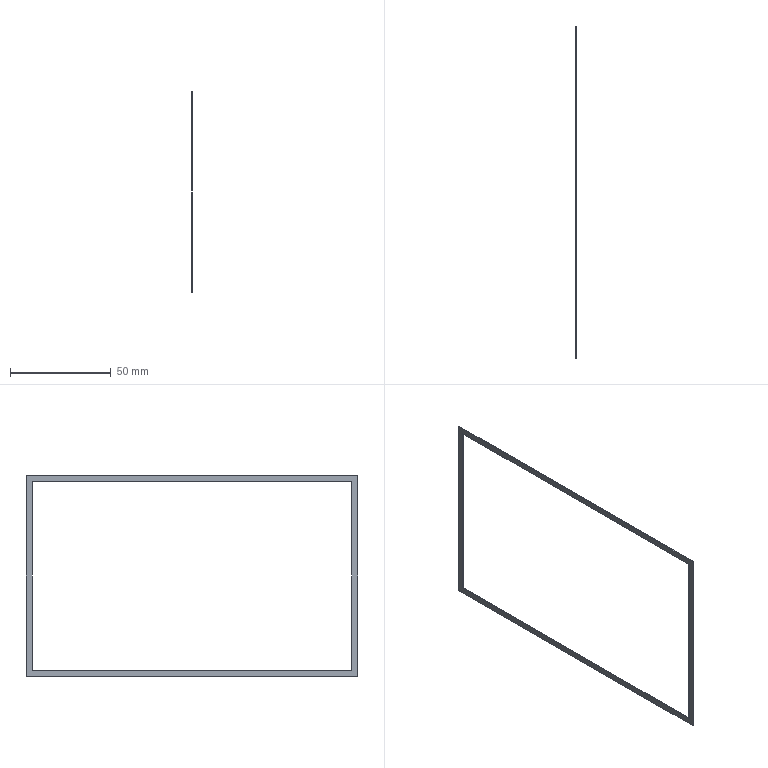Part | STEP file | 1 solid | 10 faces | box 0.3 x 164.6 x 99.7 mm | volume 464.94 mm3 | plane 10
STEP:
#1=CARTESIAN_POINT('',(0.,0.,0.));
#2=DIRECTION('',(0.,0.,1.));
#3=DIRECTION('',(1.,0.,0.));
#4=AXIS2_PLACEMENT_3D('',#1,#2,#3);
#5=CARTESIAN_POINT('',(769.075,4084.39,1378.984));
#6=VERTEX_POINT('',#5);
#7=CARTESIAN_POINT('',(769.075,4084.39,1285.284));
#8=VERTEX_POINT('',#7);
#9=CARTESIAN_POINT('',(769.075,4084.39,1378.984));
#10=DIRECTION('',(0.,0.,-1.));
#11=VECTOR('',#10,1.);
#12=LINE('',#9,#11);
#13=CARTESIAN_POINT('',(769.375,4084.39,1285.284));
#14=DIRECTION('',(0.,-1.,0.));
#15=DIRECTION('',(0.,0.,-1.));
#16=AXIS2_PLACEMENT_3D('',#13,#14,#15);
#17=PLANE('',#16);
#18=CARTESIAN_POINT('',(-93.7,-0.3));
#19=DIRECTION('',(1.,0.));
#20=VECTOR('',#19,1.);
#21=LINE('',#18,#20);
#22=(GEOMETRIC_REPRESENTATION_CONTEXT(2)PARAMETRIC_REPRESENTATION_CONTEXT()REPRESENTATION_CONTEXT('',''));
#23=DEFINITIONAL_REPRESENTATION('',(#21),#22);
#24=PCURVE('',#17,#23);
#25=CARTESIAN_POINT('',(769.075,0.,0.));
#26=DIRECTION('',(1.,0.,0.));
#27=DIRECTION('',(0.,0.,-1.));
#28=AXIS2_PLACEMENT_3D('',#25,#26,#27);
#29=PLANE('',#28);
#30=CARTESIAN_POINT('',(-1378.984,4084.39));
#31=DIRECTION('',(1.,0.));
#32=VECTOR('',#31,1.);
#33=LINE('',#30,#32);
#34=(GEOMETRIC_REPRESENTATION_CONTEXT(2)PARAMETRIC_REPRESENTATION_CONTEXT()REPRESENTATION_CONTEXT('',''));
#35=DEFINITIONAL_REPRESENTATION('',(#33),#34);
#36=PCURVE('',#29,#35);
#37=SURFACE_CURVE('',#12,(#24,#36),.PCURVE_S1.);
#38=EDGE_CURVE('',#6,#8,#37,.T.);
#39=ORIENTED_EDGE('',*,*,#38,.T.);
#40=CARTESIAN_POINT('',(769.375,4084.39,1285.284));
#41=VERTEX_POINT('',#40);
#42=CARTESIAN_POINT('',(769.075,4084.39,1285.284));
#43=DIRECTION('',(1.,0.,0.));
#44=VECTOR('',#43,1.);
#45=LINE('',#42,#44);
#46=CARTESIAN_POINT('',(0.,-0.3));
#47=DIRECTION('',(0.,1.));
#48=VECTOR('',#47,1.);
#49=LINE('',#46,#48);
#50=(GEOMETRIC_REPRESENTATION_CONTEXT(2)PARAMETRIC_REPRESENTATION_CONTEXT()REPRESENTATION_CONTEXT('',''));
#51=DEFINITIONAL_REPRESENTATION('',(#49),#50);
#52=PCURVE('',#17,#51);
#53=CARTESIAN_POINT('',(769.375,4242.99,1285.284));
#54=DIRECTION('',(0.,0.,-1.));
#55=DIRECTION('',(-1.,0.,0.));
#56=AXIS2_PLACEMENT_3D('',#53,#54,#55);
#57=PLANE('',#56);
#58=CARTESIAN_POINT('',(0.3,-158.6));
#59=DIRECTION('',(-1.,0.));
#60=VECTOR('',#59,1.);
#61=LINE('',#58,#60);
#62=(GEOMETRIC_REPRESENTATION_CONTEXT(2)PARAMETRIC_REPRESENTATION_CONTEXT()REPRESENTATION_CONTEXT('',''));
#63=DEFINITIONAL_REPRESENTATION('',(#61),#62);
#64=PCURVE('',#57,#63);
#65=SURFACE_CURVE('',#45,(#52,#64),.PCURVE_S1.);
#66=EDGE_CURVE('',#8,#41,#65,.T.);
#67=ORIENTED_EDGE('',*,*,#66,.T.);
#68=CARTESIAN_POINT('',(769.375,4084.39,1378.984));
#69=VERTEX_POINT('',#68);
#70=CARTESIAN_POINT('',(769.375,4084.39,1378.984));
#71=DIRECTION('',(0.,0.,-1.));
#72=VECTOR('',#71,1.);
#73=LINE('',#70,#72);
#74=CARTESIAN_POINT('',(-93.7,0.));
#75=DIRECTION('',(1.,0.));
#76=VECTOR('',#75,1.);
#77=LINE('',#74,#76);
#78=(GEOMETRIC_REPRESENTATION_CONTEXT(2)PARAMETRIC_REPRESENTATION_CONTEXT()REPRESENTATION_CONTEXT('',''));
#79=DEFINITIONAL_REPRESENTATION('',(#77),#78);
#80=PCURVE('',#17,#79);
#81=CARTESIAN_POINT('',(769.375,0.,0.));
#82=DIRECTION('',(1.,0.,0.));
#83=DIRECTION('',(0.,0.,-1.));
#84=AXIS2_PLACEMENT_3D('',#81,#82,#83);
#85=PLANE('',#84);
#86=CARTESIAN_POINT('',(-1378.984,4084.39));
#87=DIRECTION('',(1.,0.));
#88=VECTOR('',#87,1.);
#89=LINE('',#86,#88);
#90=(GEOMETRIC_REPRESENTATION_CONTEXT(2)PARAMETRIC_REPRESENTATION_CONTEXT()REPRESENTATION_CONTEXT('',''));
#91=DEFINITIONAL_REPRESENTATION('',(#89),#90);
#92=PCURVE('',#85,#91);
#93=SURFACE_CURVE('',#73,(#80,#92),.PCURVE_S1.);
#94=EDGE_CURVE('',#69,#41,#93,.T.);
#95=ORIENTED_EDGE('',*,*,#94,.F.);
#96=CARTESIAN_POINT('',(769.075,4084.39,1378.984));
#97=DIRECTION('',(1.,0.,0.));
#98=VECTOR('',#97,1.);
#99=LINE('',#96,#98);
#100=CARTESIAN_POINT('',(-93.7,-0.3));
#101=DIRECTION('',(0.,1.));
#102=VECTOR('',#101,1.);
#103=LINE('',#100,#102);
#104=(GEOMETRIC_REPRESENTATION_CONTEXT(2)PARAMETRIC_REPRESENTATION_CONTEXT()REPRESENTATION_CONTEXT('',''));
#105=DEFINITIONAL_REPRESENTATION('',(#103),#104);
#106=PCURVE('',#17,#105);
#107=CARTESIAN_POINT('',(769.375,4084.39,1378.984));
#108=DIRECTION('',(0.,0.,1.));
#109=DIRECTION('',(1.,0.,0.));
#110=AXIS2_PLACEMENT_3D('',#107,#108,#109);
#111=PLANE('',#110);
#112=CARTESIAN_POINT('',(-0.3,0.));
#113=DIRECTION('',(1.,0.));
#114=VECTOR('',#113,1.);
#115=LINE('',#112,#114);
#116=(GEOMETRIC_REPRESENTATION_CONTEXT(2)PARAMETRIC_REPRESENTATION_CONTEXT()REPRESENTATION_CONTEXT('',''));
#117=DEFINITIONAL_REPRESENTATION('',(#115),#116);
#118=PCURVE('',#111,#117);
#119=SURFACE_CURVE('',#99,(#106,#118),.PCURVE_S1.);
#120=EDGE_CURVE('',#6,#69,#119,.T.);
#121=ORIENTED_EDGE('',*,*,#120,.F.);
#122=EDGE_LOOP('',(#39,#67,#95,#121));
#123=FACE_BOUND('',#122,.F.);
#124=ADVANCED_FACE('',(#123),#17,.F.);
#125=CARTESIAN_POINT('',(769.075,4081.39,1282.284));
#126=VERTEX_POINT('',#125);
#127=CARTESIAN_POINT('',(769.075,4081.39,1381.984));
#128=VERTEX_POINT('',#127);
#129=CARTESIAN_POINT('',(769.075,4081.39,1282.284));
#130=DIRECTION('',(0.,0.,1.));
#131=VECTOR('',#130,1.);
#132=LINE('',#129,#131);
#133=CARTESIAN_POINT('',(-1282.284,4081.39));
#134=DIRECTION('',(-1.,0.));
#135=VECTOR('',#134,1.);
#136=LINE('',#133,#135);
#137=(GEOMETRIC_REPRESENTATION_CONTEXT(2)PARAMETRIC_REPRESENTATION_CONTEXT()REPRESENTATION_CONTEXT('',''));
#138=DEFINITIONAL_REPRESENTATION('',(#136),#137);
#139=PCURVE('',#29,#138);
#140=CARTESIAN_POINT('',(769.375,4081.39,1381.984));
#141=DIRECTION('',(0.,1.,0.));
#142=DIRECTION('',(0.,0.,1.));
#143=AXIS2_PLACEMENT_3D('',#140,#141,#142);
#144=PLANE('',#143);
#145=CARTESIAN_POINT('',(-99.7,-0.3));
#146=DIRECTION('',(1.,0.));
#147=VECTOR('',#146,1.);
#148=LINE('',#145,#147);
#149=(GEOMETRIC_REPRESENTATION_CONTEXT(2)PARAMETRIC_REPRESENTATION_CONTEXT()REPRESENTATION_CONTEXT('',''));
#150=DEFINITIONAL_REPRESENTATION('',(#148),#149);
#151=PCURVE('',#144,#150);
#152=SURFACE_CURVE('',#132,(#139,#151),.PCURVE_S1.);
#153=EDGE_CURVE('',#126,#128,#152,.T.);
#154=ORIENTED_EDGE('',*,*,#153,.F.);
#155=CARTESIAN_POINT('',(769.075,4245.99,1282.284));
#156=VERTEX_POINT('',#155);
#157=CARTESIAN_POINT('',(769.075,4245.99,1282.284));
#158=DIRECTION('',(0.,-1.,0.));
#159=VECTOR('',#158,1.);
#160=LINE('',#157,#159);
#161=CARTESIAN_POINT('',(-1282.284,4245.99));
#162=DIRECTION('',(0.,-1.));
#163=VECTOR('',#162,1.);
#164=LINE('',#161,#163);
#165=(GEOMETRIC_REPRESENTATION_CONTEXT(2)PARAMETRIC_REPRESENTATION_CONTEXT()REPRESENTATION_CONTEXT('',''));
#166=DEFINITIONAL_REPRESENTATION('',(#164),#165);
#167=PCURVE('',#29,#166);
#168=CARTESIAN_POINT('',(769.375,4081.39,1282.284));
#169=DIRECTION('',(0.,0.,1.));
#170=DIRECTION('',(1.,0.,0.));
#171=AXIS2_PLACEMENT_3D('',#168,#169,#170);
#172=PLANE('',#171);
#173=CARTESIAN_POINT('',(-0.3,164.6));
#174=DIRECTION('',(0.,-1.));
#175=VECTOR('',#174,1.);
#176=LINE('',#173,#175);
#177=(GEOMETRIC_REPRESENTATION_CONTEXT(2)PARAMETRIC_REPRESENTATION_CONTEXT()REPRESENTATION_CONTEXT('',''));
#178=DEFINITIONAL_REPRESENTATION('',(#176),#177);
#179=PCURVE('',#172,#178);
#180=SURFACE_CURVE('',#160,(#167,#179),.PCURVE_S1.);
#181=EDGE_CURVE('',#156,#126,#180,.T.);
#182=ORIENTED_EDGE('',*,*,#181,.F.);
#183=CARTESIAN_POINT('',(769.075,4245.99,1381.984));
#184=VERTEX_POINT('',#183);
#185=CARTESIAN_POINT('',(769.075,4245.99,1381.984));
#186=DIRECTION('',(0.,0.,-1.));
#187=VECTOR('',#186,1.);
#188=LINE('',#185,#187);
#189=CARTESIAN_POINT('',(-1381.984,4245.99));
#190=DIRECTION('',(1.,0.));
#191=VECTOR('',#190,1.);
#192=LINE('',#189,#191);
#193=(GEOMETRIC_REPRESENTATION_CONTEXT(2)PARAMETRIC_REPRESENTATION_CONTEXT()REPRESENTATION_CONTEXT('',''));
#194=DEFINITIONAL_REPRESENTATION('',(#192),#193);
#195=PCURVE('',#29,#194);
#196=CARTESIAN_POINT('',(769.375,4245.99,1282.284));
#197=DIRECTION('',(0.,-1.,0.));
#198=DIRECTION('',(0.,0.,-1.));
#199=AXIS2_PLACEMENT_3D('',#196,#197,#198);
#200=PLANE('',#199);
#201=CARTESIAN_POINT('',(-99.7,-0.3));
#202=DIRECTION('',(1.,0.));
#203=VECTOR('',#202,1.);
#204=LINE('',#201,#203);
#205=(GEOMETRIC_REPRESENTATION_CONTEXT(2)PARAMETRIC_REPRESENTATION_CONTEXT()REPRESENTATION_CONTEXT('',''));
#206=DEFINITIONAL_REPRESENTATION('',(#204),#205);
#207=PCURVE('',#200,#206);
#208=SURFACE_CURVE('',#188,(#195,#207),.PCURVE_S1.);
#209=EDGE_CURVE('',#184,#156,#208,.T.);
#210=ORIENTED_EDGE('',*,*,#209,.F.);
#211=CARTESIAN_POINT('',(769.075,4081.39,1381.984));
#212=DIRECTION('',(0.,1.,0.));
#213=VECTOR('',#212,1.);
#214=LINE('',#211,#213);
#215=CARTESIAN_POINT('',(-1381.984,4081.39));
#216=DIRECTION('',(0.,1.));
#217=VECTOR('',#216,1.);
#218=LINE('',#215,#217);
#219=(GEOMETRIC_REPRESENTATION_CONTEXT(2)PARAMETRIC_REPRESENTATION_CONTEXT()REPRESENTATION_CONTEXT('',''));
#220=DEFINITIONAL_REPRESENTATION('',(#218),#219);
#221=PCURVE('',#29,#220);
#222=CARTESIAN_POINT('',(769.375,4245.99,1381.984));
#223=DIRECTION('',(0.,0.,-1.));
#224=DIRECTION('',(-1.,0.,0.));
#225=AXIS2_PLACEMENT_3D('',#222,#223,#224);
#226=PLANE('',#225);
#227=CARTESIAN_POINT('',(0.3,-164.6));
#228=DIRECTION('',(0.,1.));
#229=VECTOR('',#228,1.);
#230=LINE('',#227,#229);
#231=(GEOMETRIC_REPRESENTATION_CONTEXT(2)PARAMETRIC_REPRESENTATION_CONTEXT()REPRESENTATION_CONTEXT('',''));
#232=DEFINITIONAL_REPRESENTATION('',(#230),#231);
#233=PCURVE('',#226,#232);
#234=SURFACE_CURVE('',#214,(#221,#233),.PCURVE_S1.);
#235=EDGE_CURVE('',#128,#184,#234,.T.);
#236=ORIENTED_EDGE('',*,*,#235,.F.);
#237=EDGE_LOOP('',(#154,#182,#210,#236));
#238=FACE_BOUND('',#237,.F.);
#239=ORIENTED_EDGE('',*,*,#38,.F.);
#240=CARTESIAN_POINT('',(769.075,4242.99,1378.984));
#241=VERTEX_POINT('',#240);
#242=CARTESIAN_POINT('',(769.075,4242.99,1378.984));
#243=DIRECTION('',(0.,-1.,0.));
#244=VECTOR('',#243,1.);
#245=LINE('',#242,#244);
#246=CARTESIAN_POINT('',(-1378.984,4242.99));
#247=DIRECTION('',(0.,-1.));
#248=VECTOR('',#247,1.);
#249=LINE('',#246,#248);
#250=(GEOMETRIC_REPRESENTATION_CONTEXT(2)PARAMETRIC_REPRESENTATION_CONTEXT()REPRESENTATION_CONTEXT('',''));
#251=DEFINITIONAL_REPRESENTATION('',(#249),#250);
#252=PCURVE('',#29,#251);
#253=CARTESIAN_POINT('',(-0.3,158.6));
#254=DIRECTION('',(0.,-1.));
#255=VECTOR('',#254,1.);
#256=LINE('',#253,#255);
#257=(GEOMETRIC_REPRESENTATION_CONTEXT(2)PARAMETRIC_REPRESENTATION_CONTEXT()REPRESENTATION_CONTEXT('',''));
#258=DEFINITIONAL_REPRESENTATION('',(#256),#257);
#259=PCURVE('',#111,#258);
#260=SURFACE_CURVE('',#245,(#252,#259),.PCURVE_S1.);
#261=EDGE_CURVE('',#241,#6,#260,.T.);
#262=ORIENTED_EDGE('',*,*,#261,.F.);
#263=CARTESIAN_POINT('',(769.075,4242.99,1285.284));
#264=VERTEX_POINT('',#263);
#265=CARTESIAN_POINT('',(769.075,4242.99,1285.284));
#266=DIRECTION('',(0.,0.,1.));
#267=VECTOR('',#266,1.);
#268=LINE('',#265,#267);
#269=CARTESIAN_POINT('',(-1285.284,4242.99));
#270=DIRECTION('',(-1.,0.));
#271=VECTOR('',#270,1.);
#272=LINE('',#269,#271);
#273=(GEOMETRIC_REPRESENTATION_CONTEXT(2)PARAMETRIC_REPRESENTATION_CONTEXT()REPRESENTATION_CONTEXT('',''));
#274=DEFINITIONAL_REPRESENTATION('',(#272),#273);
#275=PCURVE('',#29,#274);
#276=CARTESIAN_POINT('',(769.375,4242.99,1378.984));
#277=DIRECTION('',(0.,1.,0.));
#278=DIRECTION('',(0.,0.,1.));
#279=AXIS2_PLACEMENT_3D('',#276,#277,#278);
#280=PLANE('',#279);
#281=CARTESIAN_POINT('',(-93.7,-0.3));
#282=DIRECTION('',(1.,0.));
#283=VECTOR('',#282,1.);
#284=LINE('',#281,#283);
#285=(GEOMETRIC_REPRESENTATION_CONTEXT(2)PARAMETRIC_REPRESENTATION_CONTEXT()REPRESENTATION_CONTEXT('',''));
#286=DEFINITIONAL_REPRESENTATION('',(#284),#285);
#287=PCURVE('',#280,#286);
#288=SURFACE_CURVE('',#268,(#275,#287),.PCURVE_S1.);
#289=EDGE_CURVE('',#264,#241,#288,.T.);
#290=ORIENTED_EDGE('',*,*,#289,.F.);
#291=CARTESIAN_POINT('',(769.075,4084.39,1285.284));
#292=DIRECTION('',(0.,1.,0.));
#293=VECTOR('',#292,1.);
#294=LINE('',#291,#293);
#295=CARTESIAN_POINT('',(-1285.284,4084.39));
#296=DIRECTION('',(0.,1.));
#297=VECTOR('',#296,1.);
#298=LINE('',#295,#297);
#299=(GEOMETRIC_REPRESENTATION_CONTEXT(2)PARAMETRIC_REPRESENTATION_CONTEXT()REPRESENTATION_CONTEXT('',''));
#300=DEFINITIONAL_REPRESENTATION('',(#298),#299);
#301=PCURVE('',#29,#300);
#302=CARTESIAN_POINT('',(0.3,-158.6));
#303=DIRECTION('',(0.,1.));
#304=VECTOR('',#303,1.);
#305=LINE('',#302,#304);
#306=(GEOMETRIC_REPRESENTATION_CONTEXT(2)PARAMETRIC_REPRESENTATION_CONTEXT()REPRESENTATION_CONTEXT('',''));
#307=DEFINITIONAL_REPRESENTATION('',(#305),#306);
#308=PCURVE('',#57,#307);
#309=SURFACE_CURVE('',#294,(#301,#308),.PCURVE_S1.);
#310=EDGE_CURVE('',#8,#264,#309,.T.);
#311=ORIENTED_EDGE('',*,*,#310,.F.);
#312=EDGE_LOOP('',(#239,#262,#290,#311));
#313=FACE_BOUND('',#312,.F.);
#314=ADVANCED_FACE('',(#238,#313),#29,.F.);
#315=ORIENTED_EDGE('',*,*,#153,.T.);
#316=CARTESIAN_POINT('',(769.375,4081.39,1381.984));
#317=VERTEX_POINT('',#316);
#318=CARTESIAN_POINT('',(769.075,4081.39,1381.984));
#319=DIRECTION('',(1.,0.,0.));
#320=VECTOR('',#319,1.);
#321=LINE('',#318,#320);
#322=CARTESIAN_POINT('',(0.,-0.3));
#323=DIRECTION('',(0.,1.));
#324=VECTOR('',#323,1.);
#325=LINE('',#322,#324);
#326=(GEOMETRIC_REPRESENTATION_CONTEXT(2)PARAMETRIC_REPRESENTATION_CONTEXT()REPRESENTATION_CONTEXT('',''));
#327=DEFINITIONAL_REPRESENTATION('',(#325),#326);
#328=PCURVE('',#144,#327);
#329=CARTESIAN_POINT('',(0.3,-164.6));
#330=DIRECTION('',(-1.,0.));
#331=VECTOR('',#330,1.);
#332=LINE('',#329,#331);
#333=(GEOMETRIC_REPRESENTATION_CONTEXT(2)PARAMETRIC_REPRESENTATION_CONTEXT()REPRESENTATION_CONTEXT('',''));
#334=DEFINITIONAL_REPRESENTATION('',(#332),#333);
#335=PCURVE('',#226,#334);
#336=SURFACE_CURVE('',#321,(#328,#335),.PCURVE_S1.);
#337=EDGE_CURVE('',#128,#317,#336,.T.);
#338=ORIENTED_EDGE('',*,*,#337,.T.);
#339=CARTESIAN_POINT('',(769.375,4081.39,1282.284));
#340=VERTEX_POINT('',#339);
#341=CARTESIAN_POINT('',(769.375,4081.39,1282.284));
#342=DIRECTION('',(0.,0.,1.));
#343=VECTOR('',#342,1.);
#344=LINE('',#341,#343);
#345=CARTESIAN_POINT('',(-99.7,0.));
#346=DIRECTION('',(1.,0.));
#347=VECTOR('',#346,1.);
#348=LINE('',#345,#347);
#349=(GEOMETRIC_REPRESENTATION_CONTEXT(2)PARAMETRIC_REPRESENTATION_CONTEXT()REPRESENTATION_CONTEXT('',''));
#350=DEFINITIONAL_REPRESENTATION('',(#348),#349);
#351=PCURVE('',#144,#350);
#352=CARTESIAN_POINT('',(-1282.284,4081.39));
#353=DIRECTION('',(-1.,0.));
#354=VECTOR('',#353,1.);
#355=LINE('',#352,#354);
#356=(GEOMETRIC_REPRESENTATION_CONTEXT(2)PARAMETRIC_REPRESENTATION_CONTEXT()REPRESENTATION_CONTEXT('',''));
#357=DEFINITIONAL_REPRESENTATION('',(#355),#356);
#358=PCURVE('',#85,#357);
#359=SURFACE_CURVE('',#344,(#351,#358),.PCURVE_S1.);
#360=EDGE_CURVE('',#340,#317,#359,.T.);
#361=ORIENTED_EDGE('',*,*,#360,.F.);
#362=CARTESIAN_POINT('',(769.075,4081.39,1282.284));
#363=DIRECTION('',(1.,0.,0.));
#364=VECTOR('',#363,1.);
#365=LINE('',#362,#364);
#366=CARTESIAN_POINT('',(-99.7,-0.3));
#367=DIRECTION('',(0.,1.));
#368=VECTOR('',#367,1.);
#369=LINE('',#366,#368);
#370=(GEOMETRIC_REPRESENTATION_CONTEXT(2)PARAMETRIC_REPRESENTATION_CONTEXT()REPRESENTATION_CONTEXT('',''));
#371=DEFINITIONAL_REPRESENTATION('',(#369),#370);
#372=PCURVE('',#144,#371);
#373=CARTESIAN_POINT('',(-0.3,0.));
#374=DIRECTION('',(1.,0.));
#375=VECTOR('',#374,1.);
#376=LINE('',#373,#375);
#377=(GEOMETRIC_REPRESENTATION_CONTEXT(2)PARAMETRIC_REPRESENTATION_CONTEXT()REPRESENTATION_CONTEXT('',''));
#378=DEFINITIONAL_REPRESENTATION('',(#376),#377);
#379=PCURVE('',#172,#378);
#380=SURFACE_CURVE('',#365,(#372,#379),.PCURVE_S1.);
#381=EDGE_CURVE('',#126,#340,#380,.T.);
#382=ORIENTED_EDGE('',*,*,#381,.F.);
#383=EDGE_LOOP('',(#315,#338,#361,#382));
#384=FACE_BOUND('',#383,.F.);
#385=ADVANCED_FACE('',(#384),#144,.F.);
#386=ORIENTED_EDGE('',*,*,#235,.T.);
#387=CARTESIAN_POINT('',(769.375,4245.99,1381.984));
#388=VERTEX_POINT('',#387);
#389=CARTESIAN_POINT('',(769.075,4245.99,1381.984));
#390=DIRECTION('',(1.,0.,0.));
#391=VECTOR('',#390,1.);
#392=LINE('',#389,#391);
#393=CARTESIAN_POINT('',(0.3,0.));
#394=DIRECTION('',(-1.,0.));
#395=VECTOR('',#394,1.);
#396=LINE('',#393,#395);
#397=(GEOMETRIC_REPRESENTATION_CONTEXT(2)PARAMETRIC_REPRESENTATION_CONTEXT()REPRESENTATION_CONTEXT('',''));
#398=DEFINITIONAL_REPRESENTATION('',(#396),#397);
#399=PCURVE('',#226,#398);
#400=CARTESIAN_POINT('',(-99.7,-0.3));
#401=DIRECTION('',(0.,1.));
#402=VECTOR('',#401,1.);
#403=LINE('',#400,#402);
#404=(GEOMETRIC_REPRESENTATION_CONTEXT(2)PARAMETRIC_REPRESENTATION_CONTEXT()REPRESENTATION_CONTEXT('',''));
#405=DEFINITIONAL_REPRESENTATION('',(#403),#404);
#406=PCURVE('',#200,#405);
#407=SURFACE_CURVE('',#392,(#399,#406),.PCURVE_S1.);
#408=EDGE_CURVE('',#184,#388,#407,.T.);
#409=ORIENTED_EDGE('',*,*,#408,.T.);
#410=CARTESIAN_POINT('',(769.375,4081.39,1381.984));
#411=DIRECTION('',(0.,1.,0.));
#412=VECTOR('',#411,1.);
#413=LINE('',#410,#412);
#414=CARTESIAN_POINT('',(0.,-164.6));
#415=DIRECTION('',(0.,1.));
#416=VECTOR('',#415,1.);
#417=LINE('',#414,#416);
#418=(GEOMETRIC_REPRESENTATION_CONTEXT(2)PARAMETRIC_REPRESENTATION_CONTEXT()REPRESENTATION_CONTEXT('',''));
#419=DEFINITIONAL_REPRESENTATION('',(#417),#418);
#420=PCURVE('',#226,#419);
#421=CARTESIAN_POINT('',(-1381.984,4081.39));
#422=DIRECTION('',(0.,1.));
#423=VECTOR('',#422,1.);
#424=LINE('',#421,#423);
#425=(GEOMETRIC_REPRESENTATION_CONTEXT(2)PARAMETRIC_REPRESENTATION_CONTEXT()REPRESENTATION_CONTEXT('',''));
#426=DEFINITIONAL_REPRESENTATION('',(#424),#425);
#427=PCURVE('',#85,#426);
#428=SURFACE_CURVE('',#413,(#420,#427),.PCURVE_S1.);
#429=EDGE_CURVE('',#317,#388,#428,.T.);
#430=ORIENTED_EDGE('',*,*,#429,.F.);
#431=ORIENTED_EDGE('',*,*,#337,.F.);
#432=EDGE_LOOP('',(#386,#409,#430,#431));
#433=FACE_BOUND('',#432,.F.);
#434=ADVANCED_FACE('',(#433),#226,.F.);
#435=ORIENTED_EDGE('',*,*,#209,.T.);
#436=CARTESIAN_POINT('',(769.375,4245.99,1282.284));
#437=VERTEX_POINT('',#436);
#438=CARTESIAN_POINT('',(769.075,4245.99,1282.284));
#439=DIRECTION('',(1.,0.,0.));
#440=VECTOR('',#439,1.);
#441=LINE('',#438,#440);
#442=CARTESIAN_POINT('',(0.,-0.3));
#443=DIRECTION('',(0.,1.));
#444=VECTOR('',#443,1.);
#445=LINE('',#442,#444);
#446=(GEOMETRIC_REPRESENTATION_CONTEXT(2)PARAMETRIC_REPRESENTATION_CONTEXT()REPRESENTATION_CONTEXT('',''));
#447=DEFINITIONAL_REPRESENTATION('',(#445),#446);
#448=PCURVE('',#200,#447);
#449=CARTESIAN_POINT('',(-0.3,164.6));
#450=DIRECTION('',(1.,0.));
#451=VECTOR('',#450,1.);
#452=LINE('',#449,#451);
#453=(GEOMETRIC_REPRESENTATION_CONTEXT(2)PARAMETRIC_REPRESENTATION_CONTEXT()REPRESENTATION_CONTEXT('',''));
#454=DEFINITIONAL_REPRESENTATION('',(#452),#453);
#455=PCURVE('',#172,#454);
#456=SURFACE_CURVE('',#441,(#448,#455),.PCURVE_S1.);
#457=EDGE_CURVE('',#156,#437,#456,.T.);
#458=ORIENTED_EDGE('',*,*,#457,.T.);
#459=CARTESIAN_POINT('',(769.375,4245.99,1381.984));
#460=DIRECTION('',(0.,0.,-1.));
#461=VECTOR('',#460,1.);
#462=LINE('',#459,#461);
#463=CARTESIAN_POINT('',(-99.7,0.));
#464=DIRECTION('',(1.,0.));
#465=VECTOR('',#464,1.);
#466=LINE('',#463,#465);
#467=(GEOMETRIC_REPRESENTATION_CONTEXT(2)PARAMETRIC_REPRESENTATION_CONTEXT()REPRESENTATION_CONTEXT('',''));
#468=DEFINITIONAL_REPRESENTATION('',(#466),#467);
#469=PCURVE('',#200,#468);
#470=CARTESIAN_POINT('',(-1381.984,4245.99));
#471=DIRECTION('',(1.,0.));
#472=VECTOR('',#471,1.);
#473=LINE('',#470,#472);
#474=(GEOMETRIC_REPRESENTATION_CONTEXT(2)PARAMETRIC_REPRESENTATION_CONTEXT()REPRESENTATION_CONTEXT('',''));
#475=DEFINITIONAL_REPRESENTATION('',(#473),#474);
#476=PCURVE('',#85,#475);
#477=SURFACE_CURVE('',#462,(#469,#476),.PCURVE_S1.);
#478=EDGE_CURVE('',#388,#437,#477,.T.);
#479=ORIENTED_EDGE('',*,*,#478,.F.);
#480=ORIENTED_EDGE('',*,*,#408,.F.);
#481=EDGE_LOOP('',(#435,#458,#479,#480));
#482=FACE_BOUND('',#481,.F.);
#483=ADVANCED_FACE('',(#482),#200,.F.);
#484=ORIENTED_EDGE('',*,*,#181,.T.);
#485=ORIENTED_EDGE('',*,*,#381,.T.);
#486=CARTESIAN_POINT('',(769.375,4245.99,1282.284));
#487=DIRECTION('',(0.,-1.,0.));
#488=VECTOR('',#487,1.);
#489=LINE('',#486,#488);
#490=CARTESIAN_POINT('',(0.,164.6));
#491=DIRECTION('',(0.,-1.));
#492=VECTOR('',#491,1.);
#493=LINE('',#490,#492);
#494=(GEOMETRIC_REPRESENTATION_CONTEXT(2)PARAMETRIC_REPRESENTATION_CONTEXT()REPRESENTATION_CONTEXT('',''));
#495=DEFINITIONAL_REPRESENTATION('',(#493),#494);
#496=PCURVE('',#172,#495);
#497=CARTESIAN_POINT('',(-1282.284,4245.99));
#498=DIRECTION('',(0.,-1.));
#499=VECTOR('',#498,1.);
#500=LINE('',#497,#499);
#501=(GEOMETRIC_REPRESENTATION_CONTEXT(2)PARAMETRIC_REPRESENTATION_CONTEXT()REPRESENTATION_CONTEXT('',''));
#502=DEFINITIONAL_REPRESENTATION('',(#500),#501);
#503=PCURVE('',#85,#502);
#504=SURFACE_CURVE('',#489,(#496,#503),.PCURVE_S1.);
#505=EDGE_CURVE('',#437,#340,#504,.T.);
#506=ORIENTED_EDGE('',*,*,#505,.F.);
#507=ORIENTED_EDGE('',*,*,#457,.F.);
#508=EDGE_LOOP('',(#484,#485,#506,#507));
#509=FACE_BOUND('',#508,.F.);
#510=ADVANCED_FACE('',(#509),#172,.F.);
#511=ORIENTED_EDGE('',*,*,#360,.T.);
#512=ORIENTED_EDGE('',*,*,#429,.T.);
#513=ORIENTED_EDGE('',*,*,#478,.T.);
#514=ORIENTED_EDGE('',*,*,#505,.T.);
#515=EDGE_LOOP('',(#511,#512,#513,#514));
#516=FACE_BOUND('',#515,.F.);
#517=ORIENTED_EDGE('',*,*,#94,.T.);
#518=CARTESIAN_POINT('',(769.375,4242.99,1285.284));
#519=VERTEX_POINT('',#518);
#520=CARTESIAN_POINT('',(769.375,4084.39,1285.284));
#521=DIRECTION('',(0.,1.,0.));
#522=VECTOR('',#521,1.);
#523=LINE('',#520,#522);
#524=CARTESIAN_POINT('',(-1285.284,4084.39));
#525=DIRECTION('',(0.,1.));
#526=VECTOR('',#525,1.);
#527=LINE('',#524,#526);
#528=(GEOMETRIC_REPRESENTATION_CONTEXT(2)PARAMETRIC_REPRESENTATION_CONTEXT()REPRESENTATION_CONTEXT('',''));
#529=DEFINITIONAL_REPRESENTATION('',(#527),#528);
#530=PCURVE('',#85,#529);
#531=CARTESIAN_POINT('',(0.,-158.6));
#532=DIRECTION('',(0.,1.));
#533=VECTOR('',#532,1.);
#534=LINE('',#531,#533);
#535=(GEOMETRIC_REPRESENTATION_CONTEXT(2)PARAMETRIC_REPRESENTATION_CONTEXT()REPRESENTATION_CONTEXT('',''));
#536=DEFINITIONAL_REPRESENTATION('',(#534),#535);
#537=PCURVE('',#57,#536);
#538=SURFACE_CURVE('',#523,(#530,#537),.PCURVE_S1.);
#539=EDGE_CURVE('',#41,#519,#538,.T.);
#540=ORIENTED_EDGE('',*,*,#539,.T.);
#541=CARTESIAN_POINT('',(769.375,4242.99,1378.984));
#542=VERTEX_POINT('',#541);
#543=CARTESIAN_POINT('',(769.375,4242.99,1285.284));
#544=DIRECTION('',(0.,0.,1.));
#545=VECTOR('',#544,1.);
#546=LINE('',#543,#545);
#547=CARTESIAN_POINT('',(-1285.284,4242.99));
#548=DIRECTION('',(-1.,0.));
#549=VECTOR('',#548,1.);
#550=LINE('',#547,#549);
#551=(GEOMETRIC_REPRESENTATION_CONTEXT(2)PARAMETRIC_REPRESENTATION_CONTEXT()REPRESENTATION_CONTEXT('',''));
#552=DEFINITIONAL_REPRESENTATION('',(#550),#551);
#553=PCURVE('',#85,#552);
#554=CARTESIAN_POINT('',(-93.7,0.));
#555=DIRECTION('',(1.,0.));
#556=VECTOR('',#555,1.);
#557=LINE('',#554,#556);
#558=(GEOMETRIC_REPRESENTATION_CONTEXT(2)PARAMETRIC_REPRESENTATION_CONTEXT()REPRESENTATION_CONTEXT('',''));
#559=DEFINITIONAL_REPRESENTATION('',(#557),#558);
#560=PCURVE('',#280,#559);
#561=SURFACE_CURVE('',#546,(#553,#560),.PCURVE_S1.);
#562=EDGE_CURVE('',#519,#542,#561,.T.);
#563=ORIENTED_EDGE('',*,*,#562,.T.);
#564=CARTESIAN_POINT('',(769.375,4242.99,1378.984));
#565=DIRECTION('',(0.,-1.,0.));
#566=VECTOR('',#565,1.);
#567=LINE('',#564,#566);
#568=CARTESIAN_POINT('',(-1378.984,4242.99));
#569=DIRECTION('',(0.,-1.));
#570=VECTOR('',#569,1.);
#571=LINE('',#568,#570);
#572=(GEOMETRIC_REPRESENTATION_CONTEXT(2)PARAMETRIC_REPRESENTATION_CONTEXT()REPRESENTATION_CONTEXT('',''));
#573=DEFINITIONAL_REPRESENTATION('',(#571),#572);
#574=PCURVE('',#85,#573);
#575=CARTESIAN_POINT('',(0.,158.6));
#576=DIRECTION('',(0.,-1.));
#577=VECTOR('',#576,1.);
#578=LINE('',#575,#577);
#579=(GEOMETRIC_REPRESENTATION_CONTEXT(2)PARAMETRIC_REPRESENTATION_CONTEXT()REPRESENTATION_CONTEXT('',''));
#580=DEFINITIONAL_REPRESENTATION('',(#578),#579);
#581=PCURVE('',#111,#580);
#582=SURFACE_CURVE('',#567,(#574,#581),.PCURVE_S1.);
#583=EDGE_CURVE('',#542,#69,#582,.T.);
#584=ORIENTED_EDGE('',*,*,#583,.T.);
#585=EDGE_LOOP('',(#517,#540,#563,#584));
#586=FACE_BOUND('',#585,.F.);
#587=ADVANCED_FACE('',(#516,#586),#85,.T.);
#588=ORIENTED_EDGE('',*,*,#310,.T.);
#589=CARTESIAN_POINT('',(769.075,4242.99,1285.284));
#590=DIRECTION('',(1.,0.,0.));
#591=VECTOR('',#590,1.);
#592=LINE('',#589,#591);
#593=CARTESIAN_POINT('',(0.3,0.));
#594=DIRECTION('',(-1.,0.));
#595=VECTOR('',#594,1.);
#596=LINE('',#593,#595);
#597=(GEOMETRIC_REPRESENTATION_CONTEXT(2)PARAMETRIC_REPRESENTATION_CONTEXT()REPRESENTATION_CONTEXT('',''));
#598=DEFINITIONAL_REPRESENTATION('',(#596),#597);
#599=PCURVE('',#57,#598);
#600=CARTESIAN_POINT('',(-93.7,-0.3));
#601=DIRECTION('',(0.,1.));
#602=VECTOR('',#601,1.);
#603=LINE('',#600,#602);
#604=(GEOMETRIC_REPRESENTATION_CONTEXT(2)PARAMETRIC_REPRESENTATION_CONTEXT()REPRESENTATION_CONTEXT('',''));
#605=DEFINITIONAL_REPRESENTATION('',(#603),#604);
#606=PCURVE('',#280,#605);
#607=SURFACE_CURVE('',#592,(#599,#606),.PCURVE_S1.);
#608=EDGE_CURVE('',#264,#519,#607,.T.);
#609=ORIENTED_EDGE('',*,*,#608,.T.);
#610=ORIENTED_EDGE('',*,*,#539,.F.);
#611=ORIENTED_EDGE('',*,*,#66,.F.);
#612=EDGE_LOOP('',(#588,#609,#610,#611));
#613=FACE_BOUND('',#612,.F.);
#614=ADVANCED_FACE('',(#613),#57,.F.);
#615=ORIENTED_EDGE('',*,*,#289,.T.);
#616=CARTESIAN_POINT('',(769.075,4242.99,1378.984));
#617=DIRECTION('',(1.,0.,0.));
#618=VECTOR('',#617,1.);
#619=LINE('',#616,#618);
#620=CARTESIAN_POINT('',(0.,-0.3));
#621=DIRECTION('',(0.,1.));
#622=VECTOR('',#621,1.);
#623=LINE('',#620,#622);
#624=(GEOMETRIC_REPRESENTATION_CONTEXT(2)PARAMETRIC_REPRESENTATION_CONTEXT()REPRESENTATION_CONTEXT('',''));
#625=DEFINITIONAL_REPRESENTATION('',(#623),#624);
#626=PCURVE('',#280,#625);
#627=CARTESIAN_POINT('',(-0.3,158.6));
#628=DIRECTION('',(1.,0.));
#629=VECTOR('',#628,1.);
#630=LINE('',#627,#629);
#631=(GEOMETRIC_REPRESENTATION_CONTEXT(2)PARAMETRIC_REPRESENTATION_CONTEXT()REPRESENTATION_CONTEXT('',''));
#632=DEFINITIONAL_REPRESENTATION('',(#630),#631);
#633=PCURVE('',#111,#632);
#634=SURFACE_CURVE('',#619,(#626,#633),.PCURVE_S1.);
#635=EDGE_CURVE('',#241,#542,#634,.T.);
#636=ORIENTED_EDGE('',*,*,#635,.T.);
#637=ORIENTED_EDGE('',*,*,#562,.F.);
#638=ORIENTED_EDGE('',*,*,#608,.F.);
#639=EDGE_LOOP('',(#615,#636,#637,#638));
#640=FACE_BOUND('',#639,.F.);
#641=ADVANCED_FACE('',(#640),#280,.F.);
#642=ORIENTED_EDGE('',*,*,#261,.T.);
#643=ORIENTED_EDGE('',*,*,#120,.T.);
#644=ORIENTED_EDGE('',*,*,#583,.F.);
#645=ORIENTED_EDGE('',*,*,#635,.F.);
#646=EDGE_LOOP('',(#642,#643,#644,#645));
#647=FACE_BOUND('',#646,.F.);
#648=ADVANCED_FACE('',(#647),#111,.F.);
#649=CLOSED_SHELL('',(#124,#314,#385,#434,#483,#510,#587,#614,#641,#648));
#650=MANIFOLD_SOLID_BREP('',#649);
#651=(LENGTH_UNIT()NAMED_UNIT(*)SI_UNIT(.MILLI.,.METRE.));
#652=UNCERTAINTY_MEASURE_WITH_UNIT(LENGTH_MEASURE(0.0000001),#651,'','');
#653=(NAMED_UNIT(*)PLANE_ANGLE_UNIT()SI_UNIT($,.RADIAN.));
#654=(NAMED_UNIT(*)SI_UNIT($,.STERADIAN.)SOLID_ANGLE_UNIT());
#655=(GEOMETRIC_REPRESENTATION_CONTEXT(3)GLOBAL_UNCERTAINTY_ASSIGNED_CONTEXT((#652))GLOBAL_UNIT_ASSIGNED_CONTEXT((#651,#653,#654))REPRESENTATION_CONTEXT('',''));
#656=ADVANCED_BREP_SHAPE_REPRESENTATION('',(#4,#650),#655);